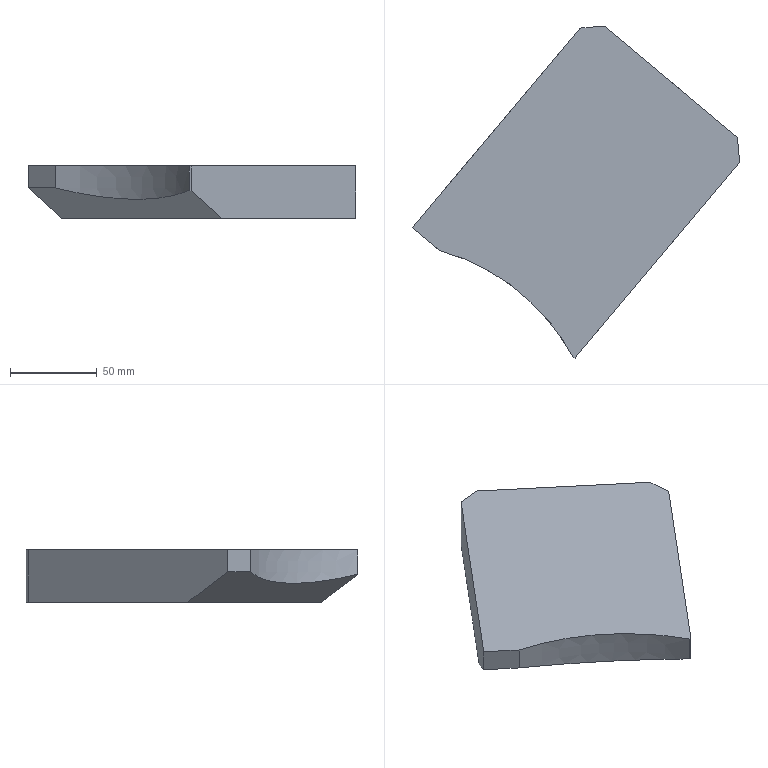Part | NX | features solid 2 | 1 solid | 13 faces | box 188.343 x 191.121 x 30 mm | volume 523826 mm3 | plane 10 | spline 1 | cone 1 | cylinder 1 | commonest cylinder face diameters 14.376 x1
STEP:
#1=CARTESIAN_POINT('',(510.282,541.788,100.));
#2=VERTEX_POINT('',#1);
#3=CARTESIAN_POINT('',(587.269,480.046,100.));
#4=VERTEX_POINT('',#3);
#5=CARTESIAN_POINT('',(510.282,541.788,100.));
#6=CARTESIAN_POINT('',(514.342,540.671,100.));
#7=CARTESIAN_POINT('',(522.327,538.042,100.));
#8=CARTESIAN_POINT('',(533.933,532.863,100.));
#9=CARTESIAN_POINT('',(545.021,526.485,100.));
#10=CARTESIAN_POINT('',(555.244,519.113,100.));
#11=CARTESIAN_POINT('',(564.691,510.717,100.));
#12=CARTESIAN_POINT('',(576.23,498.098,100.));
#13=CARTESIAN_POINT('',(583.268,487.559,100.));
#14=CARTESIAN_POINT('',(587.269,480.046,100.));
#15=B_SPLINE_CURVE_WITH_KNOTS('',3,(#5,#6,#7,#8,#9,#10,#11,#12,#13,#14),.UNSPECIFIED.,.F.,.F.,(4,1,1,1,1,1,1,4),(0.01502,0.02763,0.04025,0.05287,0.06549,0.0781,0.09072,0.116),.UNSPECIFIED.);
#16=EDGE_CURVE('',#2,#4,#15,.T.);
#17=ORIENTED_EDGE('',*,*,#16,.T.);
#18=CARTESIAN_POINT('',(588.373,479.931,100.));
#19=VERTEX_POINT('',#18);
#20=CARTESIAN_POINT('',(578.887,480.924,100.));
#21=DIRECTION('',(-0.9946,0.1042,0.));
#22=VECTOR('',#21,1000.);
#23=LINE('',#20,#22);
#24=EDGE_CURVE('',#4,#19,#23,.F.);
#25=ORIENTED_EDGE('',*,*,#24,.T.);
#26=CARTESIAN_POINT('',(682.985,592.685,100.));
#27=VERTEX_POINT('',#26);
#28=CARTESIAN_POINT('',(616.984,514.028,100.));
#29=DIRECTION('',(-0.6428,-0.766,0.));
#30=VECTOR('',#29,1000.);
#31=LINE('',#28,#30);
#32=EDGE_CURVE('',#19,#27,#31,.F.);
#33=ORIENTED_EDGE('',*,*,#32,.T.);
#34=CARTESIAN_POINT('',(681.752,606.773,100.));
#35=VERTEX_POINT('',#34);
#36=CARTESIAN_POINT('',(690.605,505.592,100.));
#37=DIRECTION('',(-0.08716,0.9962,0.));
#38=VECTOR('',#37,1000.);
#39=LINE('',#36,#38);
#40=EDGE_CURVE('',#35,#27,#39,.F.);
#41=ORIENTED_EDGE('',*,*,#40,.F.);
#42=CARTESIAN_POINT('',(605.148,671.052,100.));
#43=VERTEX_POINT('',#42);
#44=CARTESIAN_POINT('',(676.879,610.862,100.));
#45=DIRECTION('',(-0.766,0.6428,0.));
#46=VECTOR('',#45,1000.);
#47=LINE('',#44,#46);
#48=EDGE_CURVE('',#35,#43,#47,.T.);
#49=ORIENTED_EDGE('',*,*,#48,.T.);
#50=CARTESIAN_POINT('',(591.06,669.819,100.));
#51=VERTEX_POINT('',#50);
#52=CARTESIAN_POINT('',(565.446,667.578,100.));
#53=DIRECTION('',(0.9962,0.08716,0.));
#54=VECTOR('',#53,1000.);
#55=LINE('',#52,#54);
#56=EDGE_CURVE('',#51,#43,#55,.T.);
#57=ORIENTED_EDGE('',*,*,#56,.F.);
#58=CARTESIAN_POINT('',(494.642,554.913,100.));
#59=VERTEX_POINT('',#58);
#60=CARTESIAN_POINT('',(531.486,598.823,100.));
#61=DIRECTION('',(-0.6428,-0.766,0.));
#62=VECTOR('',#61,1000.);
#63=LINE('',#60,#62);
#64=EDGE_CURVE('',#59,#51,#63,.F.);
#65=ORIENTED_EDGE('',*,*,#64,.F.);
#66=CARTESIAN_POINT('',(611.463,456.888,100.));
#67=DIRECTION('',(0.766,-0.6428,0.));
#68=VECTOR('',#67,1000.);
#69=LINE('',#66,#68);
#70=EDGE_CURVE('',#59,#2,#69,.T.);
#71=ORIENTED_EDGE('',*,*,#70,.T.);
#72=EDGE_LOOP('',(#17,#25,#33,#41,#49,#57,#65,#71));
#73=FACE_BOUND('',#72,.T.);
#74=CARTESIAN_POINT('',(580.461,495.955,100.));
#75=DIRECTION('',(0.,0.,1.));
#76=DIRECTION('',(0.08716,-0.9962,0.));
#77=AXIS2_PLACEMENT_3D('',#74,#75,#76);
#78=PLANE('',#77);
#79=ADVANCED_FACE('',(#73),#78,.T.);
#80=CARTESIAN_POINT('',(510.282,541.788,87.321));
#81=VERTEX_POINT('',#80);
#82=CARTESIAN_POINT('',(510.282,541.788,87.5));
#83=DIRECTION('',(0.,0.,-1.));
#84=VECTOR('',#83,1000.);
#85=LINE('',#82,#84);
#86=EDGE_CURVE('',#2,#81,#85,.T.);
#87=ORIENTED_EDGE('',*,*,#86,.F.);
#88=ORIENTED_EDGE('',*,*,#70,.F.);
#89=CARTESIAN_POINT('',(494.642,554.913,87.321));
#90=VERTEX_POINT('',#89);
#91=CARTESIAN_POINT('',(494.642,554.913,87.5));
#92=DIRECTION('',(0.,0.,-1.));
#93=VECTOR('',#92,1000.);
#94=LINE('',#91,#93);
#95=EDGE_CURVE('',#90,#59,#94,.F.);
#96=ORIENTED_EDGE('',*,*,#95,.F.);
#97=CARTESIAN_POINT('',(599.598,466.844,87.321));
#98=DIRECTION('',(-0.766,0.6428,0.));
#99=VECTOR('',#98,1000.);
#100=LINE('',#97,#99);
#101=EDGE_CURVE('',#90,#81,#100,.F.);
#102=ORIENTED_EDGE('',*,*,#101,.T.);
#103=EDGE_LOOP('',(#87,#88,#96,#102));
#104=FACE_BOUND('',#103,.T.);
#105=CARTESIAN_POINT('',(611.463,456.888,87.5));
#106=DIRECTION('',(0.6428,0.766,0.));
#107=DIRECTION('',(0.766,-0.6428,0.));
#108=AXIS2_PLACEMENT_3D('',#105,#106,#107);
#109=PLANE('',#108);
#110=ADVANCED_FACE('',(#104),#109,.F.);
#111=CARTESIAN_POINT('',(588.373,479.931,85.698));
#112=VERTEX_POINT('',#111);
#113=CARTESIAN_POINT('',(605.85,500.759,70.));
#114=VERTEX_POINT('',#113);
#115=CARTESIAN_POINT('',(611.417,507.394,65.));
#116=DIRECTION('',(0.5567,0.6634,-0.5));
#117=VECTOR('',#116,1000.);
#118=LINE('',#115,#117);
#119=EDGE_CURVE('',#112,#114,#118,.T.);
#120=ORIENTED_EDGE('',*,*,#119,.F.);
#121=CARTESIAN_POINT('',(587.269,480.046,86.057));
#122=VERTEX_POINT('',#121);
#123=CARTESIAN_POINT('',(586.209,480.157,86.401));
#124=DIRECTION('',(-0.9464,0.09915,0.3074));
#125=VECTOR('',#124,1000.);
#126=LINE('',#123,#125);
#127=EDGE_CURVE('',#112,#122,#126,.T.);
#128=ORIENTED_EDGE('',*,*,#127,.T.);
#129=CARTESIAN_POINT('',(510.282,541.788,87.321));
#130=CARTESIAN_POINT('',(514.269,540.691,86.326));
#131=CARTESIAN_POINT('',(522.148,538.109,84.544));
#132=CARTESIAN_POINT('',(533.785,532.939,82.512));
#133=CARTESIAN_POINT('',(544.868,526.583,81.21));
#134=CARTESIAN_POINT('',(555.166,519.186,80.66));
#135=CARTESIAN_POINT('',(564.802,510.613,80.876));
#136=CARTESIAN_POINT('',(576.302,497.997,82.187));
#137=CARTESIAN_POINT('',(583.314,487.473,84.24));
#138=CARTESIAN_POINT('',(587.269,480.046,86.057));
#139=B_SPLINE_CURVE_WITH_KNOTS('',3,(#129,#130,#131,#132,#133,#134,#135,#136,#137,#138),.UNSPECIFIED.,.F.,.F.,(4,1,1,1,1,1,1,4),(0.01344,0.02619,0.03893,0.05167,0.06441,0.07716,0.0899,0.1154),.UNSPECIFIED.);
#140=EDGE_CURVE('',#81,#122,#139,.T.);
#141=ORIENTED_EDGE('',*,*,#140,.F.);
#142=ORIENTED_EDGE('',*,*,#101,.F.);
#143=CARTESIAN_POINT('',(513.925,577.894,70.));
#144=VERTEX_POINT('',#143);
#145=CARTESIAN_POINT('',(494.442,554.674,87.5));
#146=DIRECTION('',(-0.5567,-0.6634,0.5));
#147=VECTOR('',#146,1000.);
#148=LINE('',#145,#147);
#149=EDGE_CURVE('',#144,#90,#148,.T.);
#150=ORIENTED_EDGE('',*,*,#149,.F.);
#151=CARTESIAN_POINT('',(500.519,589.143,70.));
#152=DIRECTION('',(0.766,-0.6428,0.));
#153=VECTOR('',#152,1000.);
#154=LINE('',#151,#153);
#155=EDGE_CURVE('',#114,#144,#154,.F.);
#156=ORIENTED_EDGE('',*,*,#155,.F.);
#157=EDGE_LOOP('',(#120,#128,#141,#142,#150,#156));
#158=FACE_BOUND('',#157,.T.);
#159=CARTESIAN_POINT('',(599.398,466.605,87.5));
#160=DIRECTION('',(-0.3214,-0.383,-0.866));
#161=DIRECTION('',(0.8968,0.1706,-0.4082));
#162=AXIS2_PLACEMENT_3D('',#159,#160,#161);
#163=PLANE('',#162);
#164=ADVANCED_FACE('',(#158),#163,.T.);
#165=ORIENTED_EDGE('',*,*,#32,.F.);
#166=CARTESIAN_POINT('',(588.373,479.931,80.));
#167=DIRECTION('',(0.,0.,1.));
#168=VECTOR('',#167,1000.);
#169=LINE('',#166,#168);
#170=EDGE_CURVE('',#19,#112,#169,.F.);
#171=ORIENTED_EDGE('',*,*,#170,.T.);
#172=ORIENTED_EDGE('',*,*,#119,.T.);
#173=CARTESIAN_POINT('',(682.985,592.685,70.));
#174=VERTEX_POINT('',#173);
#175=CARTESIAN_POINT('',(616.984,514.028,70.));
#176=DIRECTION('',(-0.6428,-0.766,0.));
#177=VECTOR('',#176,1000.);
#178=LINE('',#175,#177);
#179=EDGE_CURVE('',#114,#174,#178,.F.);
#180=ORIENTED_EDGE('',*,*,#179,.T.);
#181=CARTESIAN_POINT('',(682.985,592.685,70.));
#182=DIRECTION('',(0.,0.,1.));
#183=VECTOR('',#182,1000.);
#184=LINE('',#181,#183);
#185=EDGE_CURVE('',#27,#174,#184,.F.);
#186=ORIENTED_EDGE('',*,*,#185,.F.);
#187=EDGE_LOOP('',(#165,#171,#172,#180,#186));
#188=FACE_BOUND('',#187,.T.);
#189=CARTESIAN_POINT('',(616.984,514.028,80.));
#190=DIRECTION('',(-0.766,0.6428,0.));
#191=DIRECTION('',(-0.6428,-0.766,0.));
#192=AXIS2_PLACEMENT_3D('',#189,#190,#191);
#193=PLANE('',#192);
#194=ADVANCED_FACE('',(#188),#193,.F.);
#195=ORIENTED_EDGE('',*,*,#179,.F.);
#196=ORIENTED_EDGE('',*,*,#155,.T.);
#197=CARTESIAN_POINT('',(591.06,669.819,70.));
#198=VERTEX_POINT('',#197);
#199=CARTESIAN_POINT('',(531.486,598.823,70.));
#200=DIRECTION('',(-0.6428,-0.766,0.));
#201=VECTOR('',#200,1000.);
#202=LINE('',#199,#201);
#203=EDGE_CURVE('',#144,#198,#202,.F.);
#204=ORIENTED_EDGE('',*,*,#203,.T.);
#205=CARTESIAN_POINT('',(605.148,671.052,70.));
#206=VERTEX_POINT('',#205);
#207=CARTESIAN_POINT('',(591.06,669.819,70.));
#208=DIRECTION('',(-0.9962,-0.08716,0.));
#209=VECTOR('',#208,1000.);
#210=LINE('',#207,#209);
#211=EDGE_CURVE('',#206,#198,#210,.T.);
#212=ORIENTED_EDGE('',*,*,#211,.F.);
#213=CARTESIAN_POINT('',(681.752,606.773,70.));
#214=VERTEX_POINT('',#213);
#215=CARTESIAN_POINT('',(584.082,688.729,70.));
#216=DIRECTION('',(-0.766,0.6428,0.));
#217=VECTOR('',#216,1000.);
#218=LINE('',#215,#217);
#219=EDGE_CURVE('',#214,#206,#218,.T.);
#220=ORIENTED_EDGE('',*,*,#219,.F.);
#221=CARTESIAN_POINT('',(681.752,606.773,70.));
#222=DIRECTION('',(0.08716,-0.9962,0.));
#223=VECTOR('',#222,1000.);
#224=LINE('',#221,#223);
#225=EDGE_CURVE('',#174,#214,#224,.F.);
#226=ORIENTED_EDGE('',*,*,#225,.F.);
#227=EDGE_LOOP('',(#195,#196,#204,#212,#220,#226));
#228=FACE_BOUND('',#227,.T.);
#229=CARTESIAN_POINT('',(487.664,573.822,70.));
#230=DIRECTION('',(0.,0.,1.));
#231=DIRECTION('',(0.08716,-0.9962,0.));
#232=AXIS2_PLACEMENT_3D('',#229,#230,#231);
#233=PLANE('',#232);
#234=ADVANCED_FACE('',(#228),#233,.F.);
#235=ORIENTED_EDGE('',*,*,#203,.F.);
#236=ORIENTED_EDGE('',*,*,#149,.T.);
#237=ORIENTED_EDGE('',*,*,#95,.T.);
#238=ORIENTED_EDGE('',*,*,#64,.T.);
#239=CARTESIAN_POINT('',(591.06,669.819,-20.));
#240=DIRECTION('',(0.,0.,-1.));
#241=VECTOR('',#240,1000.);
#242=LINE('',#239,#241);
#243=EDGE_CURVE('',#198,#51,#242,.F.);
#244=ORIENTED_EDGE('',*,*,#243,.F.);
#245=EDGE_LOOP('',(#235,#236,#237,#238,#244));
#246=FACE_BOUND('',#245,.T.);
#247=CARTESIAN_POINT('',(531.486,598.823,-20.));
#248=DIRECTION('',(-0.766,0.6428,0.));
#249=DIRECTION('',(0.6428,0.766,0.));
#250=AXIS2_PLACEMENT_3D('',#247,#248,#249);
#251=PLANE('',#250);
#252=ADVANCED_FACE('',(#246),#251,.T.);
#253=CARTESIAN_POINT('',(648.957,634.292,85.));
#254=VERTEX_POINT('',#253);
#255=CARTESIAN_POINT('',(643.45,638.912,85.));
#256=DIRECTION('',(-0.6428,-0.766,0.));
#257=DIRECTION('',(0.766,-0.6428,0.));
#258=AXIS2_PLACEMENT_3D('',#255,#256,#257);
#259=CIRCLE('',#258,7.188);
#260=EDGE_CURVE('',#254,#254,#259,.T.);
#261=ORIENTED_EDGE('',*,*,#260,.T.);
#262=EDGE_LOOP('',(#261));
#263=FACE_BOUND('',#262,.T.);
#264=ORIENTED_EDGE('',*,*,#219,.T.);
#265=CARTESIAN_POINT('',(605.148,671.052,95.));
#266=DIRECTION('',(0.,0.,-1.));
#267=VECTOR('',#266,1000.);
#268=LINE('',#265,#267);
#269=EDGE_CURVE('',#43,#206,#268,.T.);
#270=ORIENTED_EDGE('',*,*,#269,.F.);
#271=ORIENTED_EDGE('',*,*,#48,.F.);
#272=CARTESIAN_POINT('',(681.752,606.773,100.));
#273=DIRECTION('',(0.,0.,1.));
#274=VECTOR('',#273,1000.);
#275=LINE('',#272,#274);
#276=EDGE_CURVE('',#214,#35,#275,.T.);
#277=ORIENTED_EDGE('',*,*,#276,.F.);
#278=EDGE_LOOP('',(#264,#270,#271,#277));
#279=FACE_BOUND('',#278,.T.);
#280=CARTESIAN_POINT('',(584.082,688.729,95.));
#281=DIRECTION('',(-0.6428,-0.766,0.));
#282=DIRECTION('',(-0.766,0.6428,0.));
#283=AXIS2_PLACEMENT_3D('',#280,#281,#282);
#284=PLANE('',#283);
#285=ADVANCED_FACE('',(#263,#279),#284,.F.);
#286=ORIENTED_EDGE('',*,*,#225,.T.);
#287=ORIENTED_EDGE('',*,*,#276,.T.);
#288=ORIENTED_EDGE('',*,*,#40,.T.);
#289=ORIENTED_EDGE('',*,*,#185,.T.);
#290=EDGE_LOOP('',(#286,#287,#288,#289));
#291=FACE_BOUND('',#290,.T.);
#292=CARTESIAN_POINT('',(681.752,606.773,95.));
#293=DIRECTION('',(-0.9962,-0.08716,0.));
#294=DIRECTION('',(-0.08716,0.9962,0.));
#295=AXIS2_PLACEMENT_3D('',#292,#293,#294);
#296=PLANE('',#295);
#297=ADVANCED_FACE('',(#291),#296,.F.);
#298=ORIENTED_EDGE('',*,*,#211,.T.);
#299=ORIENTED_EDGE('',*,*,#243,.T.);
#300=ORIENTED_EDGE('',*,*,#56,.T.);
#301=ORIENTED_EDGE('',*,*,#269,.T.);
#302=EDGE_LOOP('',(#298,#299,#300,#301));
#303=FACE_BOUND('',#302,.T.);
#304=CARTESIAN_POINT('',(591.06,669.819,-20.));
#305=DIRECTION('',(-0.08716,0.9962,0.));
#306=DIRECTION('',(0.9962,0.08716,0.));
#307=AXIS2_PLACEMENT_3D('',#304,#305,#306);
#308=PLANE('',#307);
#309=ADVANCED_FACE('',(#303),#308,.T.);
#310=ORIENTED_EDGE('',*,*,#140,.T.);
#311=CARTESIAN_POINT('',(587.269,480.046,86.057));
#312=DIRECTION('',(0.,0.,-1.));
#313=VECTOR('',#312,1000.);
#314=LINE('',#311,#313);
#315=EDGE_CURVE('',#122,#4,#314,.F.);
#316=ORIENTED_EDGE('',*,*,#315,.T.);
#317=ORIENTED_EDGE('',*,*,#16,.F.);
#318=ORIENTED_EDGE('',*,*,#86,.T.);
#319=EDGE_LOOP('',(#310,#316,#317,#318));
#320=FACE_BOUND('',#319,.T.);
#321=CARTESIAN_POINT('',(587.269,480.046,100.));
#322=CARTESIAN_POINT('',(587.269,480.046,93.436));
#323=CARTESIAN_POINT('',(587.269,480.046,86.871));
#324=CARTESIAN_POINT('',(587.269,480.046,80.307));
#325=CARTESIAN_POINT('',(585.009,484.297,100.));
#326=CARTESIAN_POINT('',(585.009,484.297,93.436));
#327=CARTESIAN_POINT('',(585.009,484.297,86.871));
#328=CARTESIAN_POINT('',(585.009,484.297,80.307));
#329=CARTESIAN_POINT('',(580.609,491.53,100.));
#330=CARTESIAN_POINT('',(580.609,491.53,93.436));
#331=CARTESIAN_POINT('',(580.609,491.53,86.871));
#332=CARTESIAN_POINT('',(580.609,491.53,80.307));
#333=CARTESIAN_POINT('',(573.415,501.063,100.));
#334=CARTESIAN_POINT('',(573.415,501.063,93.436));
#335=CARTESIAN_POINT('',(573.415,501.063,86.871));
#336=CARTESIAN_POINT('',(573.415,501.063,80.307));
#337=CARTESIAN_POINT('',(566.83,508.412,100.));
#338=CARTESIAN_POINT('',(566.83,508.412,93.436));
#339=CARTESIAN_POINT('',(566.83,508.412,86.871));
#340=CARTESIAN_POINT('',(566.83,508.412,80.307));
#341=CARTESIAN_POINT('',(560.243,514.728,100.));
#342=CARTESIAN_POINT('',(560.243,514.728,93.436));
#343=CARTESIAN_POINT('',(560.243,514.728,86.871));
#344=CARTESIAN_POINT('',(560.243,514.728,80.307));
#345=CARTESIAN_POINT('',(553.09,520.693,100.));
#346=CARTESIAN_POINT('',(553.09,520.693,93.436));
#347=CARTESIAN_POINT('',(553.09,520.693,86.871));
#348=CARTESIAN_POINT('',(553.09,520.693,80.307));
#349=CARTESIAN_POINT('',(544.342,526.881,100.));
#350=CARTESIAN_POINT('',(544.342,526.881,93.436));
#351=CARTESIAN_POINT('',(544.342,526.881,86.871));
#352=CARTESIAN_POINT('',(544.342,526.881,80.307));
#353=CARTESIAN_POINT('',(534.59,532.482,100.));
#354=CARTESIAN_POINT('',(534.59,532.482,93.436));
#355=CARTESIAN_POINT('',(534.59,532.482,86.871));
#356=CARTESIAN_POINT('',(534.59,532.482,80.307));
#357=CARTESIAN_POINT('',(523.099,537.746,100.));
#358=CARTESIAN_POINT('',(523.099,537.746,93.436));
#359=CARTESIAN_POINT('',(523.099,537.746,86.871));
#360=CARTESIAN_POINT('',(523.099,537.746,80.307));
#361=CARTESIAN_POINT('',(515.015,540.489,100.));
#362=CARTESIAN_POINT('',(515.015,540.489,93.436));
#363=CARTESIAN_POINT('',(515.015,540.489,86.871));
#364=CARTESIAN_POINT('',(515.015,540.489,80.307));
#365=CARTESIAN_POINT('',(510.282,541.788,100.));
#366=CARTESIAN_POINT('',(510.282,541.788,93.436));
#367=CARTESIAN_POINT('',(510.282,541.788,86.871));
#368=CARTESIAN_POINT('',(510.282,541.788,80.307));
#369=B_SPLINE_SURFACE_WITH_KNOTS('',3,3,((#321,#322,#323,#324),(#325,#326,#327,#328),(#329,#330,#331,#332),(#333,#334,#335,#336),(#337,#338,#339,#340),(#341,#342,#343,#344),(#345,#346,#347,#348),(#349,#350,#351,#352),(#353,#354,#355,#356),(#357,#358,#359,#360),(#361,#362,#363,#364),(#365,#366,#367,#368)),.UNSPECIFIED.,.F.,.F.,.F.,(4,1,1,1,1,1,1,1,1,4),(4,4),(0.3386,0.3933,0.4324,0.4715,0.5027,0.534,0.573,0.6199,0.659,0.7137),(0.4443,0.5143),.UNSPECIFIED.);
#370=ADVANCED_FACE('',(#320),#369,.T.);
#371=ORIENTED_EDGE('',*,*,#24,.F.);
#372=ORIENTED_EDGE('',*,*,#315,.F.);
#373=ORIENTED_EDGE('',*,*,#127,.F.);
#374=ORIENTED_EDGE('',*,*,#170,.F.);
#375=EDGE_LOOP('',(#371,#372,#373,#374));
#376=FACE_BOUND('',#375,.T.);
#377=CARTESIAN_POINT('',(588.373,479.931,93.137));
#378=DIRECTION('',(0.1042,0.9946,0.));
#379=DIRECTION('',(-0.9946,0.1042,0.));
#380=AXIS2_PLACEMENT_3D('',#377,#378,#379);
#381=PLANE('',#380);
#382=ADVANCED_FACE('',(#376),#381,.F.);
#383=CARTESIAN_POINT('',(626.459,607.48,85.));
#384=VERTEX_POINT('',#383);
#385=CARTESIAN_POINT('',(620.953,612.101,85.));
#386=DIRECTION('',(-0.6428,-0.766,0.));
#387=DIRECTION('',(0.766,-0.6428,0.));
#388=AXIS2_PLACEMENT_3D('',#385,#386,#387);
#389=CIRCLE('',#388,7.188);
#390=EDGE_CURVE('',#384,#384,#389,.T.);
#391=ORIENTED_EDGE('',*,*,#390,.F.);
#392=EDGE_LOOP('',(#391));
#393=FACE_BOUND('',#392,.T.);
#394=CARTESIAN_POINT('',(618.176,608.792,85.));
#395=VERTEX_POINT('',#394);
#396=VERTEX_LOOP('',#395);
#397=FACE_BOUND('',#396,.T.);
#398=CARTESIAN_POINT('',(620.953,612.101,85.));
#399=DIRECTION('',(0.6428,0.766,0.));
#400=DIRECTION('',(-0.766,0.6428,0.));
#401=AXIS2_PLACEMENT_3D('',#398,#399,#400);
#402=CONICAL_SURFACE('',#401,7.188,1.03);
#403=ADVANCED_FACE('',(#393,#397),#402,.F.);
#404=ORIENTED_EDGE('',*,*,#390,.T.);
#405=EDGE_LOOP('',(#404));
#406=FACE_BOUND('',#405,.T.);
#407=ORIENTED_EDGE('',*,*,#260,.F.);
#408=EDGE_LOOP('',(#407));
#409=FACE_BOUND('',#408,.T.);
#410=CARTESIAN_POINT('',(643.45,638.912,85.));
#411=DIRECTION('',(-0.6428,-0.766,0.));
#412=DIRECTION('',(0.766,-0.6428,0.));
#413=AXIS2_PLACEMENT_3D('',#410,#411,#412);
#414=CYLINDRICAL_SURFACE('',#413,7.188);
#415=ADVANCED_FACE('',(#406,#409),#414,.F.);
#416=CLOSED_SHELL('',(#79,#110,#164,#194,#234,#252,#285,#297,#309,#370,#382,#403,#415));
#417=MANIFOLD_SOLID_BREP('',#416);
#418=(LENGTH_UNIT()NAMED_UNIT(*)SI_UNIT(.MILLI.,.METRE.));
#419=UNCERTAINTY_MEASURE_WITH_UNIT(LENGTH_MEASURE(0.0508),#418,'','');
#420=(NAMED_UNIT(*)PLANE_ANGLE_UNIT()SI_UNIT($,.RADIAN.));
#421=(NAMED_UNIT(*)SI_UNIT($,.STERADIAN.)SOLID_ANGLE_UNIT());
#422=(GEOMETRIC_REPRESENTATION_CONTEXT(3)GLOBAL_UNCERTAINTY_ASSIGNED_CONTEXT((#419))GLOBAL_UNIT_ASSIGNED_CONTEXT((#418,#420,#421))REPRESENTATION_CONTEXT('',''));
#423=ADVANCED_BREP_SHAPE_REPRESENTATION('',(#417),#422);